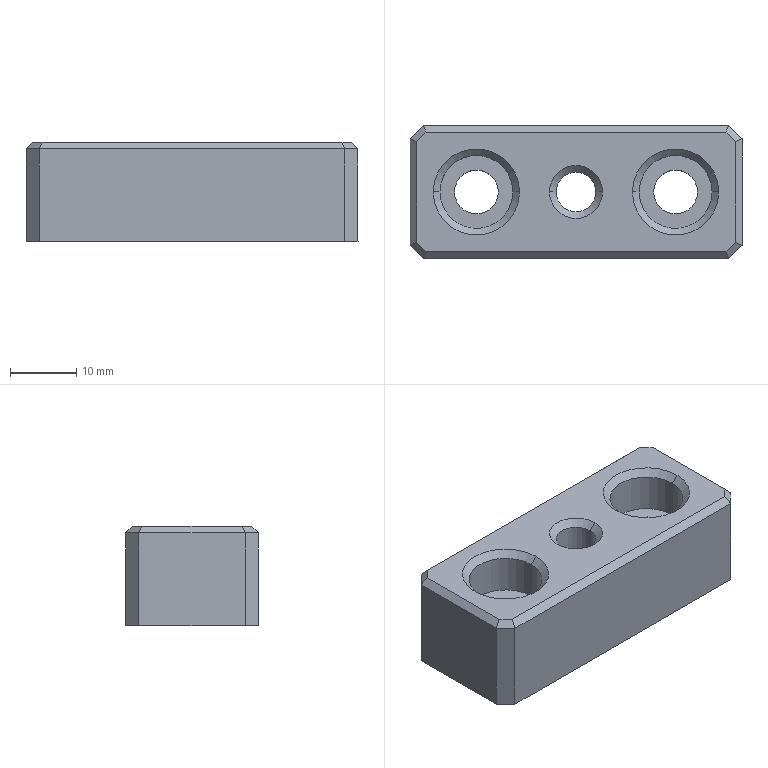Part | SolidWorks | features BaseBody 1 | 1 solid | 36 faces | box 50 x 20 x 15 mm | volume 12489 mm3 | plane 20 | cylinder 10 | cone 6 | commonest cylinder face diameters 6.6 x4 11 x4 6 x2
STEP:
#1=CARTESIAN_POINT('',(360.247,467.,-346.345));
#2=VERTEX_POINT('',#1);
#3=CARTESIAN_POINT('',(354.247,467.,-346.345));
#4=VERTEX_POINT('',#3);
#5=CARTESIAN_POINT('',(357.247,467.,-346.345));
#6=DIRECTION('',(0.,0.,-1.));
#7=DIRECTION('',(-1.,0.,0.));
#8=AXIS2_PLACEMENT_3D('',#5,#6,#7);
#9=CIRCLE('',#8,3.);
#10=EDGE_CURVE('',#2,#4,#9,.T.);
#11=ORIENTED_EDGE('',*,*,#10,.F.);
#12=CARTESIAN_POINT('',(360.247,467.,-360.345));
#13=VERTEX_POINT('',#12);
#14=CARTESIAN_POINT('',(360.247,467.,-360.345));
#15=DIRECTION('',(0.,0.,-1.));
#16=VECTOR('',#15,1000.);
#17=LINE('',#14,#16);
#18=EDGE_CURVE('',#2,#13,#17,.T.);
#19=ORIENTED_EDGE('',*,*,#18,.T.);
#20=CARTESIAN_POINT('',(354.247,467.,-360.345));
#21=VERTEX_POINT('',#20);
#22=CARTESIAN_POINT('',(357.247,467.,-360.345));
#23=DIRECTION('',(0.,0.,-1.));
#24=DIRECTION('',(-1.,0.,0.));
#25=AXIS2_PLACEMENT_3D('',#22,#23,#24);
#26=CIRCLE('',#25,3.);
#27=EDGE_CURVE('',#13,#21,#26,.T.);
#28=ORIENTED_EDGE('',*,*,#27,.T.);
#29=CARTESIAN_POINT('',(354.247,467.,-360.345));
#30=DIRECTION('',(0.,0.,-1.));
#31=VECTOR('',#30,1000.);
#32=LINE('',#29,#31);
#33=EDGE_CURVE('',#4,#21,#32,.T.);
#34=ORIENTED_EDGE('',*,*,#33,.F.);
#35=EDGE_LOOP('',(#11,#19,#28,#34));
#36=FACE_OUTER_BOUND('',#35,.T.);
#37=CARTESIAN_POINT('',(357.247,467.,-360.345));
#38=DIRECTION('',(0.,0.,-1.));
#39=DIRECTION('',(-1.,0.,0.));
#40=AXIS2_PLACEMENT_3D('',#37,#38,#39);
#41=CYLINDRICAL_SURFACE('',#40,3.);
#42=ADVANCED_FACE('',(#36),#41,.F.);
#43=CARTESIAN_POINT('',(345.547,467.,-360.345));
#44=VERTEX_POINT('',#43);
#45=CARTESIAN_POINT('',(338.947,467.,-360.345));
#46=VERTEX_POINT('',#45);
#47=CARTESIAN_POINT('',(342.247,467.,-360.345));
#48=DIRECTION('',(0.,0.,-1.));
#49=DIRECTION('',(1.,0.,0.));
#50=AXIS2_PLACEMENT_3D('',#47,#48,#49);
#51=CIRCLE('',#50,3.3);
#52=EDGE_CURVE('',#44,#46,#51,.T.);
#53=ORIENTED_EDGE('',*,*,#52,.T.);
#54=CARTESIAN_POINT('',(338.947,467.,-352.145));
#55=VERTEX_POINT('',#54);
#56=CARTESIAN_POINT('',(338.947,467.,-345.345));
#57=DIRECTION('',(0.,0.,1.));
#58=VECTOR('',#57,1000.);
#59=LINE('',#56,#58);
#60=EDGE_CURVE('',#46,#55,#59,.T.);
#61=ORIENTED_EDGE('',*,*,#60,.T.);
#62=CARTESIAN_POINT('',(345.547,467.,-352.145));
#63=VERTEX_POINT('',#62);
#64=CARTESIAN_POINT('',(342.247,467.,-352.145));
#65=DIRECTION('',(0.,0.,-1.));
#66=DIRECTION('',(1.,0.,0.));
#67=AXIS2_PLACEMENT_3D('',#64,#65,#66);
#68=CIRCLE('',#67,3.3);
#69=EDGE_CURVE('',#63,#55,#68,.T.);
#70=ORIENTED_EDGE('',*,*,#69,.F.);
#71=CARTESIAN_POINT('',(345.547,467.,-345.345));
#72=DIRECTION('',(0.,0.,1.));
#73=VECTOR('',#72,1000.);
#74=LINE('',#71,#73);
#75=EDGE_CURVE('',#44,#63,#74,.T.);
#76=ORIENTED_EDGE('',*,*,#75,.F.);
#77=EDGE_LOOP('',(#53,#61,#70,#76));
#78=FACE_OUTER_BOUND('',#77,.T.);
#79=CARTESIAN_POINT('',(342.247,467.,-345.345));
#80=DIRECTION('',(0.,0.,1.));
#81=DIRECTION('',(1.,0.,0.));
#82=AXIS2_PLACEMENT_3D('',#79,#80,#81);
#83=CYLINDRICAL_SURFACE('',#82,3.3);
#84=ADVANCED_FACE('',(#78),#83,.F.);
#85=CARTESIAN_POINT('',(375.547,467.,-360.345));
#86=VERTEX_POINT('',#85);
#87=CARTESIAN_POINT('',(368.947,467.,-360.345));
#88=VERTEX_POINT('',#87);
#89=CARTESIAN_POINT('',(372.247,467.,-360.345));
#90=DIRECTION('',(0.,0.,-1.));
#91=DIRECTION('',(1.,0.,0.));
#92=AXIS2_PLACEMENT_3D('',#89,#90,#91);
#93=CIRCLE('',#92,3.3);
#94=EDGE_CURVE('',#86,#88,#93,.T.);
#95=ORIENTED_EDGE('',*,*,#94,.T.);
#96=CARTESIAN_POINT('',(368.947,467.,-352.145));
#97=VERTEX_POINT('',#96);
#98=CARTESIAN_POINT('',(368.947,467.,-345.345));
#99=DIRECTION('',(0.,0.,1.));
#100=VECTOR('',#99,1000.);
#101=LINE('',#98,#100);
#102=EDGE_CURVE('',#88,#97,#101,.T.);
#103=ORIENTED_EDGE('',*,*,#102,.T.);
#104=CARTESIAN_POINT('',(375.547,467.,-352.145));
#105=VERTEX_POINT('',#104);
#106=CARTESIAN_POINT('',(372.247,467.,-352.145));
#107=DIRECTION('',(0.,0.,-1.));
#108=DIRECTION('',(1.,0.,0.));
#109=AXIS2_PLACEMENT_3D('',#106,#107,#108);
#110=CIRCLE('',#109,3.3);
#111=EDGE_CURVE('',#105,#97,#110,.T.);
#112=ORIENTED_EDGE('',*,*,#111,.F.);
#113=CARTESIAN_POINT('',(375.547,467.,-345.345));
#114=DIRECTION('',(0.,0.,1.));
#115=VECTOR('',#114,1000.);
#116=LINE('',#113,#115);
#117=EDGE_CURVE('',#86,#105,#116,.T.);
#118=ORIENTED_EDGE('',*,*,#117,.F.);
#119=EDGE_LOOP('',(#95,#103,#112,#118));
#120=FACE_OUTER_BOUND('',#119,.T.);
#121=CARTESIAN_POINT('',(372.247,467.,-345.345));
#122=DIRECTION('',(0.,0.,1.));
#123=DIRECTION('',(1.,0.,0.));
#124=AXIS2_PLACEMENT_3D('',#121,#122,#123);
#125=CYLINDRICAL_SURFACE('',#124,3.3);
#126=ADVANCED_FACE('',(#120),#125,.F.);
#127=ORIENTED_EDGE('',*,*,#10,.T.);
#128=CARTESIAN_POINT('',(353.247,467.,-345.345));
#129=VERTEX_POINT('',#128);
#130=CARTESIAN_POINT('',(353.247,467.,-345.345));
#131=DIRECTION('',(-0.7071,0.,0.7071));
#132=VECTOR('',#131,1000.);
#133=LINE('',#130,#132);
#134=EDGE_CURVE('',#4,#129,#133,.T.);
#135=ORIENTED_EDGE('',*,*,#134,.T.);
#136=CARTESIAN_POINT('',(361.247,467.,-345.345));
#137=VERTEX_POINT('',#136);
#138=CARTESIAN_POINT('',(357.247,467.,-345.345));
#139=DIRECTION('',(0.,0.,-1.));
#140=DIRECTION('',(1.,0.,0.));
#141=AXIS2_PLACEMENT_3D('',#138,#139,#140);
#142=CIRCLE('',#141,4.);
#143=EDGE_CURVE('',#137,#129,#142,.T.);
#144=ORIENTED_EDGE('',*,*,#143,.F.);
#145=CARTESIAN_POINT('',(361.247,467.,-345.345));
#146=DIRECTION('',(0.7071,0.,0.7071));
#147=VECTOR('',#146,1000.);
#148=LINE('',#145,#147);
#149=EDGE_CURVE('',#2,#137,#148,.T.);
#150=ORIENTED_EDGE('',*,*,#149,.F.);
#151=EDGE_LOOP('',(#127,#135,#144,#150));
#152=FACE_OUTER_BOUND('',#151,.T.);
#153=CARTESIAN_POINT('',(357.247,467.,-345.345));
#154=DIRECTION('',(0.,0.,1.));
#155=DIRECTION('',(1.,0.,0.));
#156=AXIS2_PLACEMENT_3D('',#153,#154,#155);
#157=CONICAL_SURFACE('',#156,4.,0.7854);
#158=ADVANCED_FACE('',(#152),#157,.F.);
#159=CARTESIAN_POINT('',(347.747,467.,-352.145));
#160=VERTEX_POINT('',#159);
#161=CARTESIAN_POINT('',(336.747,467.,-352.145));
#162=VERTEX_POINT('',#161);
#163=CARTESIAN_POINT('',(342.247,467.,-352.145));
#164=DIRECTION('',(0.,0.,-1.));
#165=DIRECTION('',(1.,0.,0.));
#166=AXIS2_PLACEMENT_3D('',#163,#164,#165);
#167=CIRCLE('',#166,5.5);
#168=EDGE_CURVE('',#160,#162,#167,.T.);
#169=ORIENTED_EDGE('',*,*,#168,.T.);
#170=CARTESIAN_POINT('',(336.747,467.,-346.345));
#171=VERTEX_POINT('',#170);
#172=CARTESIAN_POINT('',(336.747,467.,-345.345));
#173=DIRECTION('',(0.,0.,1.));
#174=VECTOR('',#173,1000.);
#175=LINE('',#172,#174);
#176=EDGE_CURVE('',#162,#171,#175,.T.);
#177=ORIENTED_EDGE('',*,*,#176,.T.);
#178=CARTESIAN_POINT('',(347.747,467.,-346.345));
#179=VERTEX_POINT('',#178);
#180=CARTESIAN_POINT('',(342.247,467.,-346.345));
#181=DIRECTION('',(0.,0.,-1.));
#182=DIRECTION('',(1.,0.,0.));
#183=AXIS2_PLACEMENT_3D('',#180,#181,#182);
#184=CIRCLE('',#183,5.5);
#185=EDGE_CURVE('',#179,#171,#184,.T.);
#186=ORIENTED_EDGE('',*,*,#185,.F.);
#187=CARTESIAN_POINT('',(347.747,467.,-345.345));
#188=DIRECTION('',(0.,0.,1.));
#189=VECTOR('',#188,1000.);
#190=LINE('',#187,#189);
#191=EDGE_CURVE('',#160,#179,#190,.T.);
#192=ORIENTED_EDGE('',*,*,#191,.F.);
#193=EDGE_LOOP('',(#169,#177,#186,#192));
#194=FACE_OUTER_BOUND('',#193,.T.);
#195=CARTESIAN_POINT('',(342.247,467.,-345.345));
#196=DIRECTION('',(0.,0.,1.));
#197=DIRECTION('',(1.,0.,0.));
#198=AXIS2_PLACEMENT_3D('',#195,#196,#197);
#199=CYLINDRICAL_SURFACE('',#198,5.5);
#200=ADVANCED_FACE('',(#194),#199,.F.);
#201=CARTESIAN_POINT('',(377.747,467.,-352.145));
#202=VERTEX_POINT('',#201);
#203=CARTESIAN_POINT('',(366.747,467.,-352.145));
#204=VERTEX_POINT('',#203);
#205=CARTESIAN_POINT('',(372.247,467.,-352.145));
#206=DIRECTION('',(0.,0.,-1.));
#207=DIRECTION('',(1.,0.,0.));
#208=AXIS2_PLACEMENT_3D('',#205,#206,#207);
#209=CIRCLE('',#208,5.5);
#210=EDGE_CURVE('',#202,#204,#209,.T.);
#211=ORIENTED_EDGE('',*,*,#210,.T.);
#212=CARTESIAN_POINT('',(366.747,467.,-346.345));
#213=VERTEX_POINT('',#212);
#214=CARTESIAN_POINT('',(366.747,467.,-345.345));
#215=DIRECTION('',(0.,0.,1.));
#216=VECTOR('',#215,1000.);
#217=LINE('',#214,#216);
#218=EDGE_CURVE('',#204,#213,#217,.T.);
#219=ORIENTED_EDGE('',*,*,#218,.T.);
#220=CARTESIAN_POINT('',(377.747,467.,-346.345));
#221=VERTEX_POINT('',#220);
#222=CARTESIAN_POINT('',(372.247,467.,-346.345));
#223=DIRECTION('',(0.,0.,-1.));
#224=DIRECTION('',(1.,0.,0.));
#225=AXIS2_PLACEMENT_3D('',#222,#223,#224);
#226=CIRCLE('',#225,5.5);
#227=EDGE_CURVE('',#221,#213,#226,.T.);
#228=ORIENTED_EDGE('',*,*,#227,.F.);
#229=CARTESIAN_POINT('',(377.747,467.,-345.345));
#230=DIRECTION('',(0.,0.,1.));
#231=VECTOR('',#230,1000.);
#232=LINE('',#229,#231);
#233=EDGE_CURVE('',#202,#221,#232,.T.);
#234=ORIENTED_EDGE('',*,*,#233,.F.);
#235=EDGE_LOOP('',(#211,#219,#228,#234));
#236=FACE_OUTER_BOUND('',#235,.T.);
#237=CARTESIAN_POINT('',(372.247,467.,-345.345));
#238=DIRECTION('',(0.,0.,1.));
#239=DIRECTION('',(1.,0.,0.));
#240=AXIS2_PLACEMENT_3D('',#237,#238,#239);
#241=CYLINDRICAL_SURFACE('',#240,5.5);
#242=ADVANCED_FACE('',(#236),#241,.F.);
#243=ORIENTED_EDGE('',*,*,#227,.T.);
#244=CARTESIAN_POINT('',(365.747,467.,-345.345));
#245=VERTEX_POINT('',#244);
#246=CARTESIAN_POINT('',(365.747,467.,-345.345));
#247=DIRECTION('',(-0.7071,0.,0.7071));
#248=VECTOR('',#247,1000.);
#249=LINE('',#246,#248);
#250=EDGE_CURVE('',#213,#245,#249,.T.);
#251=ORIENTED_EDGE('',*,*,#250,.T.);
#252=CARTESIAN_POINT('',(378.747,467.,-345.345));
#253=VERTEX_POINT('',#252);
#254=CARTESIAN_POINT('',(372.247,467.,-345.345));
#255=DIRECTION('',(0.,0.,-1.));
#256=DIRECTION('',(1.,0.,0.));
#257=AXIS2_PLACEMENT_3D('',#254,#255,#256);
#258=CIRCLE('',#257,6.5);
#259=EDGE_CURVE('',#253,#245,#258,.T.);
#260=ORIENTED_EDGE('',*,*,#259,.F.);
#261=CARTESIAN_POINT('',(378.747,467.,-345.345));
#262=DIRECTION('',(0.7071,0.,0.7071));
#263=VECTOR('',#262,1000.);
#264=LINE('',#261,#263);
#265=EDGE_CURVE('',#221,#253,#264,.T.);
#266=ORIENTED_EDGE('',*,*,#265,.F.);
#267=EDGE_LOOP('',(#243,#251,#260,#266));
#268=FACE_OUTER_BOUND('',#267,.T.);
#269=CARTESIAN_POINT('',(372.247,467.,-345.345));
#270=DIRECTION('',(0.,0.,1.));
#271=DIRECTION('',(1.,0.,0.));
#272=AXIS2_PLACEMENT_3D('',#269,#270,#271);
#273=CONICAL_SURFACE('',#272,6.5,0.7854);
#274=ADVANCED_FACE('',(#268),#273,.F.);
#275=ORIENTED_EDGE('',*,*,#185,.T.);
#276=CARTESIAN_POINT('',(335.747,467.,-345.345));
#277=VERTEX_POINT('',#276);
#278=CARTESIAN_POINT('',(335.747,467.,-345.345));
#279=DIRECTION('',(-0.7071,0.,0.7071));
#280=VECTOR('',#279,1000.);
#281=LINE('',#278,#280);
#282=EDGE_CURVE('',#171,#277,#281,.T.);
#283=ORIENTED_EDGE('',*,*,#282,.T.);
#284=CARTESIAN_POINT('',(348.747,467.,-345.345));
#285=VERTEX_POINT('',#284);
#286=CARTESIAN_POINT('',(342.247,467.,-345.345));
#287=DIRECTION('',(0.,0.,-1.));
#288=DIRECTION('',(1.,0.,0.));
#289=AXIS2_PLACEMENT_3D('',#286,#287,#288);
#290=CIRCLE('',#289,6.5);
#291=EDGE_CURVE('',#285,#277,#290,.T.);
#292=ORIENTED_EDGE('',*,*,#291,.F.);
#293=CARTESIAN_POINT('',(348.747,467.,-345.345));
#294=DIRECTION('',(0.7071,0.,0.7071));
#295=VECTOR('',#294,1000.);
#296=LINE('',#293,#295);
#297=EDGE_CURVE('',#179,#285,#296,.T.);
#298=ORIENTED_EDGE('',*,*,#297,.F.);
#299=EDGE_LOOP('',(#275,#283,#292,#298));
#300=FACE_OUTER_BOUND('',#299,.T.);
#301=CARTESIAN_POINT('',(342.247,467.,-345.345));
#302=DIRECTION('',(0.,0.,1.));
#303=DIRECTION('',(1.,0.,0.));
#304=AXIS2_PLACEMENT_3D('',#301,#302,#303);
#305=CONICAL_SURFACE('',#304,6.5,0.7854);
#306=ADVANCED_FACE('',(#300),#305,.F.);
#307=CARTESIAN_POINT('',(357.247,467.,-360.345));
#308=DIRECTION('',(0.,0.,-1.));
#309=DIRECTION('',(-1.,0.,0.));
#310=AXIS2_PLACEMENT_3D('',#307,#308,#309);
#311=CIRCLE('',#310,3.);
#312=EDGE_CURVE('',#21,#13,#311,.T.);
#313=ORIENTED_EDGE('',*,*,#312,.F.);
#314=ORIENTED_EDGE('',*,*,#27,.F.);
#315=EDGE_LOOP('',(#313,#314));
#316=FACE_BOUND('',#315,.T.);
#317=ORIENTED_EDGE('',*,*,#52,.F.);
#318=CARTESIAN_POINT('',(342.247,467.,-360.345));
#319=DIRECTION('',(0.,0.,-1.));
#320=DIRECTION('',(1.,0.,0.));
#321=AXIS2_PLACEMENT_3D('',#318,#319,#320);
#322=CIRCLE('',#321,3.3);
#323=EDGE_CURVE('',#46,#44,#322,.T.);
#324=ORIENTED_EDGE('',*,*,#323,.F.);
#325=EDGE_LOOP('',(#317,#324));
#326=FACE_BOUND('',#325,.T.);
#327=ORIENTED_EDGE('',*,*,#94,.F.);
#328=CARTESIAN_POINT('',(372.247,467.,-360.345));
#329=DIRECTION('',(0.,0.,-1.));
#330=DIRECTION('',(1.,0.,0.));
#331=AXIS2_PLACEMENT_3D('',#328,#329,#330);
#332=CIRCLE('',#331,3.3);
#333=EDGE_CURVE('',#88,#86,#332,.T.);
#334=ORIENTED_EDGE('',*,*,#333,.F.);
#335=EDGE_LOOP('',(#327,#334));
#336=FACE_BOUND('',#335,.T.);
#337=CARTESIAN_POINT('',(332.247,475.,-360.345));
#338=VERTEX_POINT('',#337);
#339=CARTESIAN_POINT('',(332.247,459.,-360.345));
#340=VERTEX_POINT('',#339);
#341=CARTESIAN_POINT('',(332.247,467.,-360.345));
#342=DIRECTION('',(0.,-1.,0.));
#343=VECTOR('',#342,1000.);
#344=LINE('',#341,#343);
#345=EDGE_CURVE('',#338,#340,#344,.T.);
#346=ORIENTED_EDGE('',*,*,#345,.F.);
#347=CARTESIAN_POINT('',(334.247,477.,-360.345));
#348=VERTEX_POINT('',#347);
#349=CARTESIAN_POINT('',(334.247,477.,-360.345));
#350=DIRECTION('',(-0.7071,-0.7071,0.));
#351=VECTOR('',#350,1000.);
#352=LINE('',#349,#351);
#353=EDGE_CURVE('',#348,#338,#352,.T.);
#354=ORIENTED_EDGE('',*,*,#353,.F.);
#355=CARTESIAN_POINT('',(380.247,477.,-360.345));
#356=VERTEX_POINT('',#355);
#357=CARTESIAN_POINT('',(357.247,477.,-360.345));
#358=DIRECTION('',(-1.,0.,0.));
#359=VECTOR('',#358,1000.);
#360=LINE('',#357,#359);
#361=EDGE_CURVE('',#356,#348,#360,.T.);
#362=ORIENTED_EDGE('',*,*,#361,.F.);
#363=CARTESIAN_POINT('',(382.247,475.,-360.345));
#364=VERTEX_POINT('',#363);
#365=CARTESIAN_POINT('',(382.247,475.,-360.345));
#366=DIRECTION('',(-0.7071,0.7071,0.));
#367=VECTOR('',#366,1000.);
#368=LINE('',#365,#367);
#369=EDGE_CURVE('',#364,#356,#368,.T.);
#370=ORIENTED_EDGE('',*,*,#369,.F.);
#371=CARTESIAN_POINT('',(382.247,459.,-360.345));
#372=VERTEX_POINT('',#371);
#373=CARTESIAN_POINT('',(382.247,467.,-360.345));
#374=DIRECTION('',(0.,1.,0.));
#375=VECTOR('',#374,1000.);
#376=LINE('',#373,#375);
#377=EDGE_CURVE('',#372,#364,#376,.T.);
#378=ORIENTED_EDGE('',*,*,#377,.F.);
#379=CARTESIAN_POINT('',(380.247,457.,-360.345));
#380=VERTEX_POINT('',#379);
#381=CARTESIAN_POINT('',(380.247,457.,-360.345));
#382=DIRECTION('',(0.7071,0.7071,0.));
#383=VECTOR('',#382,1000.);
#384=LINE('',#381,#383);
#385=EDGE_CURVE('',#380,#372,#384,.T.);
#386=ORIENTED_EDGE('',*,*,#385,.F.);
#387=CARTESIAN_POINT('',(334.247,457.,-360.345));
#388=VERTEX_POINT('',#387);
#389=CARTESIAN_POINT('',(357.247,457.,-360.345));
#390=DIRECTION('',(1.,0.,0.));
#391=VECTOR('',#390,1000.);
#392=LINE('',#389,#391);
#393=EDGE_CURVE('',#388,#380,#392,.T.);
#394=ORIENTED_EDGE('',*,*,#393,.F.);
#395=CARTESIAN_POINT('',(332.247,459.,-360.345));
#396=DIRECTION('',(0.7071,-0.7071,0.));
#397=VECTOR('',#396,1000.);
#398=LINE('',#395,#397);
#399=EDGE_CURVE('',#340,#388,#398,.T.);
#400=ORIENTED_EDGE('',*,*,#399,.F.);
#401=EDGE_LOOP('',(#346,#354,#362,#370,#378,#386,#394,#400));
#402=FACE_OUTER_BOUND('',#401,.T.);
#403=CARTESIAN_POINT('',(357.247,467.,-360.345));
#404=DIRECTION('',(0.,0.,1.));
#405=DIRECTION('',(1.,0.,0.));
#406=AXIS2_PLACEMENT_3D('',#403,#404,#405);
#407=PLANE('',#406);
#408=ADVANCED_FACE('',(#316,#326,#336,#402),#407,.F.);
#409=ORIENTED_EDGE('',*,*,#18,.F.);
#410=CARTESIAN_POINT('',(357.247,467.,-346.345));
#411=DIRECTION('',(0.,0.,-1.));
#412=DIRECTION('',(-1.,0.,0.));
#413=AXIS2_PLACEMENT_3D('',#410,#411,#412);
#414=CIRCLE('',#413,3.);
#415=EDGE_CURVE('',#4,#2,#414,.T.);
#416=ORIENTED_EDGE('',*,*,#415,.F.);
#417=ORIENTED_EDGE('',*,*,#33,.T.);
#418=ORIENTED_EDGE('',*,*,#312,.T.);
#419=EDGE_LOOP('',(#409,#416,#417,#418));
#420=FACE_OUTER_BOUND('',#419,.T.);
#421=CARTESIAN_POINT('',(357.247,467.,-360.345));
#422=DIRECTION('',(0.,0.,-1.));
#423=DIRECTION('',(-1.,0.,0.));
#424=AXIS2_PLACEMENT_3D('',#421,#422,#423);
#425=CYLINDRICAL_SURFACE('',#424,3.);
#426=ADVANCED_FACE('',(#420),#425,.F.);
#427=ORIENTED_EDGE('',*,*,#60,.F.);
#428=ORIENTED_EDGE('',*,*,#323,.T.);
#429=ORIENTED_EDGE('',*,*,#75,.T.);
#430=CARTESIAN_POINT('',(342.247,467.,-352.145));
#431=DIRECTION('',(0.,0.,-1.));
#432=DIRECTION('',(1.,0.,0.));
#433=AXIS2_PLACEMENT_3D('',#430,#431,#432);
#434=CIRCLE('',#433,3.3);
#435=EDGE_CURVE('',#55,#63,#434,.T.);
#436=ORIENTED_EDGE('',*,*,#435,.F.);
#437=EDGE_LOOP('',(#427,#428,#429,#436));
#438=FACE_OUTER_BOUND('',#437,.T.);
#439=CARTESIAN_POINT('',(342.247,467.,-345.345));
#440=DIRECTION('',(0.,0.,1.));
#441=DIRECTION('',(1.,0.,0.));
#442=AXIS2_PLACEMENT_3D('',#439,#440,#441);
#443=CYLINDRICAL_SURFACE('',#442,3.3);
#444=ADVANCED_FACE('',(#438),#443,.F.);
#445=ORIENTED_EDGE('',*,*,#102,.F.);
#446=ORIENTED_EDGE('',*,*,#333,.T.);
#447=ORIENTED_EDGE('',*,*,#117,.T.);
#448=CARTESIAN_POINT('',(372.247,467.,-352.145));
#449=DIRECTION('',(0.,0.,-1.));
#450=DIRECTION('',(1.,0.,0.));
#451=AXIS2_PLACEMENT_3D('',#448,#449,#450);
#452=CIRCLE('',#451,3.3);
#453=EDGE_CURVE('',#97,#105,#452,.T.);
#454=ORIENTED_EDGE('',*,*,#453,.F.);
#455=EDGE_LOOP('',(#445,#446,#447,#454));
#456=FACE_OUTER_BOUND('',#455,.T.);
#457=CARTESIAN_POINT('',(372.247,467.,-345.345));
#458=DIRECTION('',(0.,0.,1.));
#459=DIRECTION('',(1.,0.,0.));
#460=AXIS2_PLACEMENT_3D('',#457,#458,#459);
#461=CYLINDRICAL_SURFACE('',#460,3.3);
#462=ADVANCED_FACE('',(#456),#461,.F.);
#463=CARTESIAN_POINT('',(332.247,459.,-346.345));
#464=VERTEX_POINT('',#463);
#465=CARTESIAN_POINT('',(332.247,459.,-345.345));
#466=DIRECTION('',(0.,0.,1.));
#467=VECTOR('',#466,1000.);
#468=LINE('',#465,#467);
#469=EDGE_CURVE('',#340,#464,#468,.T.);
#470=ORIENTED_EDGE('',*,*,#469,.F.);
#471=ORIENTED_EDGE('',*,*,#399,.T.);
#472=CARTESIAN_POINT('',(334.247,457.,-346.345));
#473=VERTEX_POINT('',#472);
#474=CARTESIAN_POINT('',(334.247,457.,-345.345));
#475=DIRECTION('',(0.,0.,-1.));
#476=VECTOR('',#475,1000.);
#477=LINE('',#474,#476);
#478=EDGE_CURVE('',#473,#388,#477,.T.);
#479=ORIENTED_EDGE('',*,*,#478,.F.);
#480=CARTESIAN_POINT('',(334.247,457.,-346.345));
#481=DIRECTION('',(0.7071,-0.7071,0.));
#482=VECTOR('',#481,1000.);
#483=LINE('',#480,#482);
#484=EDGE_CURVE('',#464,#473,#483,.T.);
#485=ORIENTED_EDGE('',*,*,#484,.F.);
#486=EDGE_LOOP('',(#470,#471,#479,#485));
#487=FACE_OUTER_BOUND('',#486,.T.);
#488=CARTESIAN_POINT('',(334.247,457.,-345.345));
#489=DIRECTION('',(0.7071,0.7071,0.));
#490=DIRECTION('',(-0.7071,0.7071,0.));
#491=AXIS2_PLACEMENT_3D('',#488,#489,#490);
#492=PLANE('',#491);
#493=ADVANCED_FACE('',(#487),#492,.F.);
#494=CARTESIAN_POINT('',(332.247,475.,-346.345));
#495=VERTEX_POINT('',#494);
#496=CARTESIAN_POINT('',(332.247,475.,-345.345));
#497=DIRECTION('',(0.,0.,1.));
#498=VECTOR('',#497,1000.);
#499=LINE('',#496,#498);
#500=EDGE_CURVE('',#338,#495,#499,.T.);
#501=ORIENTED_EDGE('',*,*,#500,.F.);
#502=ORIENTED_EDGE('',*,*,#345,.T.);
#503=ORIENTED_EDGE('',*,*,#469,.T.);
#504=CARTESIAN_POINT('',(332.247,457.,-346.345));
#505=DIRECTION('',(0.,-1.,0.));
#506=VECTOR('',#505,1000.);
#507=LINE('',#504,#506);
#508=EDGE_CURVE('',#495,#464,#507,.T.);
#509=ORIENTED_EDGE('',*,*,#508,.F.);
#510=EDGE_LOOP('',(#501,#502,#503,#509));
#511=FACE_OUTER_BOUND('',#510,.T.);
#512=CARTESIAN_POINT('',(332.247,457.,-345.345));
#513=DIRECTION('',(1.,0.,0.));
#514=DIRECTION('',(0.,0.,-1.));
#515=AXIS2_PLACEMENT_3D('',#512,#513,#514);
#516=PLANE('',#515);
#517=ADVANCED_FACE('',(#511),#516,.F.);
#518=CARTESIAN_POINT('',(334.247,477.,-346.345));
#519=VERTEX_POINT('',#518);
#520=CARTESIAN_POINT('',(334.247,477.,-345.345));
#521=DIRECTION('',(0.,0.,1.));
#522=VECTOR('',#521,1000.);
#523=LINE('',#520,#522);
#524=EDGE_CURVE('',#348,#519,#523,.T.);
#525=ORIENTED_EDGE('',*,*,#524,.F.);
#526=ORIENTED_EDGE('',*,*,#353,.T.);
#527=ORIENTED_EDGE('',*,*,#500,.T.);
#528=CARTESIAN_POINT('',(332.247,475.,-346.345));
#529=DIRECTION('',(-0.7071,-0.7071,0.));
#530=VECTOR('',#529,1000.);
#531=LINE('',#528,#530);
#532=EDGE_CURVE('',#519,#495,#531,.T.);
#533=ORIENTED_EDGE('',*,*,#532,.F.);
#534=EDGE_LOOP('',(#525,#526,#527,#533));
#535=FACE_OUTER_BOUND('',#534,.T.);
#536=CARTESIAN_POINT('',(332.247,475.,-345.345));
#537=DIRECTION('',(0.7071,-0.7071,0.));
#538=DIRECTION('',(0.7071,0.7071,0.));
#539=AXIS2_PLACEMENT_3D('',#536,#537,#538);
#540=PLANE('',#539);
#541=ADVANCED_FACE('',(#535),#540,.F.);
#542=CARTESIAN_POINT('',(380.247,477.,-346.345));
#543=VERTEX_POINT('',#542);
#544=CARTESIAN_POINT('',(380.247,477.,-345.345));
#545=DIRECTION('',(0.,0.,1.));
#546=VECTOR('',#545,1000.);
#547=LINE('',#544,#546);
#548=EDGE_CURVE('',#356,#543,#547,.T.);
#549=ORIENTED_EDGE('',*,*,#548,.F.);
#550=ORIENTED_EDGE('',*,*,#361,.T.);
#551=ORIENTED_EDGE('',*,*,#524,.T.);
#552=CARTESIAN_POINT('',(332.247,477.,-346.345));
#553=DIRECTION('',(-1.,0.,0.));
#554=VECTOR('',#553,1000.);
#555=LINE('',#552,#554);
#556=EDGE_CURVE('',#543,#519,#555,.T.);
#557=ORIENTED_EDGE('',*,*,#556,.F.);
#558=EDGE_LOOP('',(#549,#550,#551,#557));
#559=FACE_OUTER_BOUND('',#558,.T.);
#560=CARTESIAN_POINT('',(332.247,477.,-345.345));
#561=DIRECTION('',(0.,-1.,0.));
#562=DIRECTION('',(0.,0.,-1.));
#563=AXIS2_PLACEMENT_3D('',#560,#561,#562);
#564=PLANE('',#563);
#565=ADVANCED_FACE('',(#559),#564,.F.);
#566=CARTESIAN_POINT('',(382.247,475.,-346.345));
#567=VERTEX_POINT('',#566);
#568=CARTESIAN_POINT('',(382.247,475.,-345.345));
#569=DIRECTION('',(0.,0.,1.));
#570=VECTOR('',#569,1000.);
#571=LINE('',#568,#570);
#572=EDGE_CURVE('',#364,#567,#571,.T.);
#573=ORIENTED_EDGE('',*,*,#572,.F.);
#574=ORIENTED_EDGE('',*,*,#369,.T.);
#575=ORIENTED_EDGE('',*,*,#548,.T.);
#576=CARTESIAN_POINT('',(380.247,477.,-346.345));
#577=DIRECTION('',(-0.7071,0.7071,0.));
#578=VECTOR('',#577,1000.);
#579=LINE('',#576,#578);
#580=EDGE_CURVE('',#567,#543,#579,.T.);
#581=ORIENTED_EDGE('',*,*,#580,.F.);
#582=EDGE_LOOP('',(#573,#574,#575,#581));
#583=FACE_OUTER_BOUND('',#582,.T.);
#584=CARTESIAN_POINT('',(380.247,477.,-345.345));
#585=DIRECTION('',(-0.7071,-0.7071,0.));
#586=DIRECTION('',(0.7071,-0.7071,0.));
#587=AXIS2_PLACEMENT_3D('',#584,#585,#586);
#588=PLANE('',#587);
#589=ADVANCED_FACE('',(#583),#588,.F.);
#590=CARTESIAN_POINT('',(382.247,459.,-346.345));
#591=VERTEX_POINT('',#590);
#592=CARTESIAN_POINT('',(382.247,459.,-345.345));
#593=DIRECTION('',(0.,0.,1.));
#594=VECTOR('',#593,1000.);
#595=LINE('',#592,#594);
#596=EDGE_CURVE('',#372,#591,#595,.T.);
#597=ORIENTED_EDGE('',*,*,#596,.F.);
#598=ORIENTED_EDGE('',*,*,#377,.T.);
#599=ORIENTED_EDGE('',*,*,#572,.T.);
#600=CARTESIAN_POINT('',(382.247,457.,-346.345));
#601=DIRECTION('',(0.,1.,0.));
#602=VECTOR('',#601,1000.);
#603=LINE('',#600,#602);
#604=EDGE_CURVE('',#591,#567,#603,.T.);
#605=ORIENTED_EDGE('',*,*,#604,.F.);
#606=EDGE_LOOP('',(#597,#598,#599,#605));
#607=FACE_OUTER_BOUND('',#606,.T.);
#608=CARTESIAN_POINT('',(382.247,457.,-345.345));
#609=DIRECTION('',(-1.,0.,0.));
#610=DIRECTION('',(0.,0.,1.));
#611=AXIS2_PLACEMENT_3D('',#608,#609,#610);
#612=PLANE('',#611);
#613=ADVANCED_FACE('',(#607),#612,.F.);
#614=CARTESIAN_POINT('',(380.247,457.,-346.345));
#615=VERTEX_POINT('',#614);
#616=CARTESIAN_POINT('',(380.247,457.,-345.345));
#617=DIRECTION('',(0.,0.,1.));
#618=VECTOR('',#617,1000.);
#619=LINE('',#616,#618);
#620=EDGE_CURVE('',#380,#615,#619,.T.);
#621=ORIENTED_EDGE('',*,*,#620,.F.);
#622=ORIENTED_EDGE('',*,*,#385,.T.);
#623=ORIENTED_EDGE('',*,*,#596,.T.);
#624=CARTESIAN_POINT('',(382.247,459.,-346.345));
#625=DIRECTION('',(0.7071,0.7071,0.));
#626=VECTOR('',#625,1000.);
#627=LINE('',#624,#626);
#628=EDGE_CURVE('',#615,#591,#627,.T.);
#629=ORIENTED_EDGE('',*,*,#628,.F.);
#630=EDGE_LOOP('',(#621,#622,#623,#629));
#631=FACE_OUTER_BOUND('',#630,.T.);
#632=CARTESIAN_POINT('',(382.247,459.,-345.345));
#633=DIRECTION('',(-0.7071,0.7071,0.));
#634=DIRECTION('',(-0.7071,-0.7071,0.));
#635=AXIS2_PLACEMENT_3D('',#632,#633,#634);
#636=PLANE('',#635);
#637=ADVANCED_FACE('',(#631),#636,.F.);
#638=ORIENTED_EDGE('',*,*,#478,.T.);
#639=ORIENTED_EDGE('',*,*,#393,.T.);
#640=ORIENTED_EDGE('',*,*,#620,.T.);
#641=CARTESIAN_POINT('',(332.247,457.,-346.345));
#642=DIRECTION('',(1.,0.,0.));
#643=VECTOR('',#642,1000.);
#644=LINE('',#641,#643);
#645=EDGE_CURVE('',#473,#615,#644,.T.);
#646=ORIENTED_EDGE('',*,*,#645,.F.);
#647=EDGE_LOOP('',(#638,#639,#640,#646));
#648=FACE_OUTER_BOUND('',#647,.T.);
#649=CARTESIAN_POINT('',(332.247,457.,-345.345));
#650=DIRECTION('',(0.,1.,0.));
#651=DIRECTION('',(0.,0.,1.));
#652=AXIS2_PLACEMENT_3D('',#649,#650,#651);
#653=PLANE('',#652);
#654=ADVANCED_FACE('',(#648),#653,.F.);
#655=ORIENTED_EDGE('',*,*,#134,.F.);
#656=ORIENTED_EDGE('',*,*,#415,.T.);
#657=ORIENTED_EDGE('',*,*,#149,.T.);
#658=CARTESIAN_POINT('',(357.247,467.,-345.345));
#659=DIRECTION('',(0.,0.,-1.));
#660=DIRECTION('',(1.,0.,0.));
#661=AXIS2_PLACEMENT_3D('',#658,#659,#660);
#662=CIRCLE('',#661,4.);
#663=EDGE_CURVE('',#129,#137,#662,.T.);
#664=ORIENTED_EDGE('',*,*,#663,.F.);
#665=EDGE_LOOP('',(#655,#656,#657,#664));
#666=FACE_OUTER_BOUND('',#665,.T.);
#667=CARTESIAN_POINT('',(357.247,467.,-345.345));
#668=DIRECTION('',(0.,0.,1.));
#669=DIRECTION('',(1.,0.,0.));
#670=AXIS2_PLACEMENT_3D('',#667,#668,#669);
#671=CONICAL_SURFACE('',#670,4.,0.7854);
#672=ADVANCED_FACE('',(#666),#671,.F.);
#673=ORIENTED_EDGE('',*,*,#69,.T.);
#674=ORIENTED_EDGE('',*,*,#435,.T.);
#675=EDGE_LOOP('',(#673,#674));
#676=FACE_BOUND('',#675,.T.);
#677=ORIENTED_EDGE('',*,*,#168,.F.);
#678=CARTESIAN_POINT('',(342.247,467.,-352.145));
#679=DIRECTION('',(0.,0.,-1.));
#680=DIRECTION('',(1.,0.,0.));
#681=AXIS2_PLACEMENT_3D('',#678,#679,#680);
#682=CIRCLE('',#681,5.5);
#683=EDGE_CURVE('',#162,#160,#682,.T.);
#684=ORIENTED_EDGE('',*,*,#683,.F.);
#685=EDGE_LOOP('',(#677,#684));
#686=FACE_OUTER_BOUND('',#685,.T.);
#687=CARTESIAN_POINT('',(342.247,470.3,-352.145));
#688=DIRECTION('',(0.,0.,-1.));
#689=DIRECTION('',(-1.,0.,0.));
#690=AXIS2_PLACEMENT_3D('',#687,#688,#689);
#691=PLANE('',#690);
#692=ADVANCED_FACE('',(#676,#686),#691,.F.);
#693=ORIENTED_EDGE('',*,*,#111,.T.);
#694=ORIENTED_EDGE('',*,*,#453,.T.);
#695=EDGE_LOOP('',(#693,#694));
#696=FACE_BOUND('',#695,.T.);
#697=ORIENTED_EDGE('',*,*,#210,.F.);
#698=CARTESIAN_POINT('',(372.247,467.,-352.145));
#699=DIRECTION('',(0.,0.,-1.));
#700=DIRECTION('',(1.,0.,0.));
#701=AXIS2_PLACEMENT_3D('',#698,#699,#700);
#702=CIRCLE('',#701,5.5);
#703=EDGE_CURVE('',#204,#202,#702,.T.);
#704=ORIENTED_EDGE('',*,*,#703,.F.);
#705=EDGE_LOOP('',(#697,#704));
#706=FACE_OUTER_BOUND('',#705,.T.);
#707=CARTESIAN_POINT('',(372.247,470.3,-352.145));
#708=DIRECTION('',(0.,0.,-1.));
#709=DIRECTION('',(-1.,0.,0.));
#710=AXIS2_PLACEMENT_3D('',#707,#708,#709);
#711=PLANE('',#710);
#712=ADVANCED_FACE('',(#696,#706),#711,.F.);
#713=ORIENTED_EDGE('',*,*,#484,.T.);
#714=CARTESIAN_POINT('',(334.661,458.,-345.345));
#715=VERTEX_POINT('',#714);
#716=CARTESIAN_POINT('',(334.247,457.,-346.345));
#717=DIRECTION('',(0.2811,0.6786,0.6786));
#718=VECTOR('',#717,1000.);
#719=LINE('',#716,#718);
#720=EDGE_CURVE('',#473,#715,#719,.T.);
#721=ORIENTED_EDGE('',*,*,#720,.T.);
#722=CARTESIAN_POINT('',(333.247,459.414,-345.345));
#723=VERTEX_POINT('',#722);
#724=CARTESIAN_POINT('',(334.661,458.,-345.345));
#725=DIRECTION('',(-0.7071,0.7071,0.));
#726=VECTOR('',#725,1000.);
#727=LINE('',#724,#726);
#728=EDGE_CURVE('',#715,#723,#727,.T.);
#729=ORIENTED_EDGE('',*,*,#728,.T.);
#730=CARTESIAN_POINT('',(333.247,459.414,-345.345));
#731=DIRECTION('',(-0.6786,-0.2811,-0.6786));
#732=VECTOR('',#731,1000.);
#733=LINE('',#730,#732);
#734=EDGE_CURVE('',#723,#464,#733,.T.);
#735=ORIENTED_EDGE('',*,*,#734,.T.);
#736=EDGE_LOOP('',(#713,#721,#729,#735));
#737=FACE_OUTER_BOUND('',#736,.T.);
#738=CARTESIAN_POINT('',(341.454,451.207,-345.345));
#739=DIRECTION('',(-0.5,-0.5,0.7071));
#740=DIRECTION('',(0.8165,0.,0.5774));
#741=AXIS2_PLACEMENT_3D('',#738,#739,#740);
#742=PLANE('',#741);
#743=ADVANCED_FACE('',(#737),#742,.T.);
#744=ORIENTED_EDGE('',*,*,#508,.T.);
#745=ORIENTED_EDGE('',*,*,#734,.F.);
#746=CARTESIAN_POINT('',(333.247,474.586,-345.345));
#747=VERTEX_POINT('',#746);
#748=CARTESIAN_POINT('',(333.247,467.,-345.345));
#749=DIRECTION('',(0.,1.,0.));
#750=VECTOR('',#749,1000.);
#751=LINE('',#748,#750);
#752=EDGE_CURVE('',#723,#747,#751,.T.);
#753=ORIENTED_EDGE('',*,*,#752,.T.);
#754=CARTESIAN_POINT('',(333.247,474.586,-345.345));
#755=DIRECTION('',(-0.6786,0.2811,-0.6786));
#756=VECTOR('',#755,1000.);
#757=LINE('',#754,#756);
#758=EDGE_CURVE('',#747,#495,#757,.T.);
#759=ORIENTED_EDGE('',*,*,#758,.T.);
#760=EDGE_LOOP('',(#744,#745,#753,#759));
#761=FACE_OUTER_BOUND('',#760,.T.);
#762=CARTESIAN_POINT('',(333.247,467.,-345.345));
#763=DIRECTION('',(-0.7071,0.,0.7071));
#764=DIRECTION('',(0.7071,0.,0.7071));
#765=AXIS2_PLACEMENT_3D('',#762,#763,#764);
#766=PLANE('',#765);
#767=ADVANCED_FACE('',(#761),#766,.T.);
#768=CARTESIAN_POINT('',(334.661,476.,-345.345));
#769=VERTEX_POINT('',#768);
#770=CARTESIAN_POINT('',(333.247,474.586,-345.345));
#771=DIRECTION('',(0.7071,0.7071,0.));
#772=VECTOR('',#771,1000.);
#773=LINE('',#770,#772);
#774=EDGE_CURVE('',#747,#769,#773,.T.);
#775=ORIENTED_EDGE('',*,*,#774,.T.);
#776=CARTESIAN_POINT('',(334.661,476.,-345.345));
#777=DIRECTION('',(-0.2811,0.6786,-0.6786));
#778=VECTOR('',#777,1000.);
#779=LINE('',#776,#778);
#780=EDGE_CURVE('',#769,#519,#779,.T.);
#781=ORIENTED_EDGE('',*,*,#780,.T.);
#782=ORIENTED_EDGE('',*,*,#532,.T.);
#783=ORIENTED_EDGE('',*,*,#758,.F.);
#784=EDGE_LOOP('',(#775,#781,#782,#783));
#785=FACE_OUTER_BOUND('',#784,.T.);
#786=CARTESIAN_POINT('',(341.454,482.793,-345.345));
#787=DIRECTION('',(-0.5,0.5,0.7071));
#788=DIRECTION('',(0.8165,0.,0.5774));
#789=AXIS2_PLACEMENT_3D('',#786,#787,#788);
#790=PLANE('',#789);
#791=ADVANCED_FACE('',(#785),#790,.T.);
#792=CARTESIAN_POINT('',(379.832,476.,-345.345));
#793=VERTEX_POINT('',#792);
#794=CARTESIAN_POINT('',(357.247,476.,-345.345));
#795=DIRECTION('',(1.,0.,0.));
#796=VECTOR('',#795,1000.);
#797=LINE('',#794,#796);
#798=EDGE_CURVE('',#769,#793,#797,.T.);
#799=ORIENTED_EDGE('',*,*,#798,.T.);
#800=CARTESIAN_POINT('',(379.832,476.,-345.345));
#801=DIRECTION('',(0.2811,0.6786,-0.6786));
#802=VECTOR('',#801,1000.);
#803=LINE('',#800,#802);
#804=EDGE_CURVE('',#793,#543,#803,.T.);
#805=ORIENTED_EDGE('',*,*,#804,.T.);
#806=ORIENTED_EDGE('',*,*,#556,.T.);
#807=ORIENTED_EDGE('',*,*,#780,.F.);
#808=EDGE_LOOP('',(#799,#805,#806,#807));
#809=FACE_OUTER_BOUND('',#808,.T.);
#810=CARTESIAN_POINT('',(357.247,476.,-345.345));
#811=DIRECTION('',(0.,0.7071,0.7071));
#812=DIRECTION('',(0.,-0.7071,0.7071));
#813=AXIS2_PLACEMENT_3D('',#810,#811,#812);
#814=PLANE('',#813);
#815=ADVANCED_FACE('',(#809),#814,.T.);
#816=CARTESIAN_POINT('',(381.247,474.586,-345.345));
#817=VERTEX_POINT('',#816);
#818=CARTESIAN_POINT('',(379.832,476.,-345.345));
#819=DIRECTION('',(0.7071,-0.7071,0.));
#820=VECTOR('',#819,1000.);
#821=LINE('',#818,#820);
#822=EDGE_CURVE('',#793,#817,#821,.T.);
#823=ORIENTED_EDGE('',*,*,#822,.T.);
#824=CARTESIAN_POINT('',(381.247,474.586,-345.345));
#825=DIRECTION('',(0.6786,0.2811,-0.6786));
#826=VECTOR('',#825,1000.);
#827=LINE('',#824,#826);
#828=EDGE_CURVE('',#817,#567,#827,.T.);
#829=ORIENTED_EDGE('',*,*,#828,.T.);
#830=ORIENTED_EDGE('',*,*,#580,.T.);
#831=ORIENTED_EDGE('',*,*,#804,.F.);
#832=EDGE_LOOP('',(#823,#829,#830,#831));
#833=FACE_OUTER_BOUND('',#832,.T.);
#834=CARTESIAN_POINT('',(373.039,482.793,-345.345));
#835=DIRECTION('',(0.5,0.5,0.7071));
#836=DIRECTION('',(0.8165,0.,-0.5774));
#837=AXIS2_PLACEMENT_3D('',#834,#835,#836);
#838=PLANE('',#837);
#839=ADVANCED_FACE('',(#833),#838,.T.);
#840=CARTESIAN_POINT('',(381.247,459.414,-345.345));
#841=VERTEX_POINT('',#840);
#842=CARTESIAN_POINT('',(381.247,467.,-345.345));
#843=DIRECTION('',(0.,-1.,0.));
#844=VECTOR('',#843,1000.);
#845=LINE('',#842,#844);
#846=EDGE_CURVE('',#817,#841,#845,.T.);
#847=ORIENTED_EDGE('',*,*,#846,.T.);
#848=CARTESIAN_POINT('',(381.247,459.414,-345.345));
#849=DIRECTION('',(0.6786,-0.2811,-0.6786));
#850=VECTOR('',#849,1000.);
#851=LINE('',#848,#850);
#852=EDGE_CURVE('',#841,#591,#851,.T.);
#853=ORIENTED_EDGE('',*,*,#852,.T.);
#854=ORIENTED_EDGE('',*,*,#604,.T.);
#855=ORIENTED_EDGE('',*,*,#828,.F.);
#856=EDGE_LOOP('',(#847,#853,#854,#855));
#857=FACE_OUTER_BOUND('',#856,.T.);
#858=CARTESIAN_POINT('',(381.247,467.,-345.345));
#859=DIRECTION('',(0.7071,0.,0.7071));
#860=DIRECTION('',(0.7071,0.,-0.7071));
#861=AXIS2_PLACEMENT_3D('',#858,#859,#860);
#862=PLANE('',#861);
#863=ADVANCED_FACE('',(#857),#862,.T.);
#864=CARTESIAN_POINT('',(379.832,458.,-345.345));
#865=VERTEX_POINT('',#864);
#866=CARTESIAN_POINT('',(381.247,459.414,-345.345));
#867=DIRECTION('',(-0.7071,-0.7071,0.));
#868=VECTOR('',#867,1000.);
#869=LINE('',#866,#868);
#870=EDGE_CURVE('',#841,#865,#869,.T.);
#871=ORIENTED_EDGE('',*,*,#870,.T.);
#872=CARTESIAN_POINT('',(379.832,458.,-345.345));
#873=DIRECTION('',(0.2811,-0.6786,-0.6786));
#874=VECTOR('',#873,1000.);
#875=LINE('',#872,#874);
#876=EDGE_CURVE('',#865,#615,#875,.T.);
#877=ORIENTED_EDGE('',*,*,#876,.T.);
#878=ORIENTED_EDGE('',*,*,#628,.T.);
#879=ORIENTED_EDGE('',*,*,#852,.F.);
#880=EDGE_LOOP('',(#871,#877,#878,#879));
#881=FACE_OUTER_BOUND('',#880,.T.);
#882=CARTESIAN_POINT('',(373.039,451.207,-345.345));
#883=DIRECTION('',(0.5,-0.5,0.7071));
#884=DIRECTION('',(0.8165,0.,-0.5774));
#885=AXIS2_PLACEMENT_3D('',#882,#883,#884);
#886=PLANE('',#885);
#887=ADVANCED_FACE('',(#881),#886,.T.);
#888=ORIENTED_EDGE('',*,*,#645,.T.);
#889=ORIENTED_EDGE('',*,*,#876,.F.);
#890=CARTESIAN_POINT('',(357.247,458.,-345.345));
#891=DIRECTION('',(-1.,0.,0.));
#892=VECTOR('',#891,1000.);
#893=LINE('',#890,#892);
#894=EDGE_CURVE('',#865,#715,#893,.T.);
#895=ORIENTED_EDGE('',*,*,#894,.T.);
#896=ORIENTED_EDGE('',*,*,#720,.F.);
#897=EDGE_LOOP('',(#888,#889,#895,#896));
#898=FACE_OUTER_BOUND('',#897,.T.);
#899=CARTESIAN_POINT('',(357.247,458.,-345.345));
#900=DIRECTION('',(0.,-0.7071,0.7071));
#901=DIRECTION('',(0.,-0.7071,-0.7071));
#902=AXIS2_PLACEMENT_3D('',#899,#900,#901);
#903=PLANE('',#902);
#904=ADVANCED_FACE('',(#898),#903,.T.);
#905=ORIENTED_EDGE('',*,*,#143,.T.);
#906=ORIENTED_EDGE('',*,*,#663,.T.);
#907=EDGE_LOOP('',(#905,#906));
#908=FACE_BOUND('',#907,.T.);
#909=ORIENTED_EDGE('',*,*,#259,.T.);
#910=CARTESIAN_POINT('',(372.247,467.,-345.345));
#911=DIRECTION('',(0.,0.,-1.));
#912=DIRECTION('',(1.,0.,0.));
#913=AXIS2_PLACEMENT_3D('',#910,#911,#912);
#914=CIRCLE('',#913,6.5);
#915=EDGE_CURVE('',#245,#253,#914,.T.);
#916=ORIENTED_EDGE('',*,*,#915,.T.);
#917=EDGE_LOOP('',(#909,#916));
#918=FACE_BOUND('',#917,.T.);
#919=ORIENTED_EDGE('',*,*,#291,.T.);
#920=CARTESIAN_POINT('',(342.247,467.,-345.345));
#921=DIRECTION('',(0.,0.,-1.));
#922=DIRECTION('',(1.,0.,0.));
#923=AXIS2_PLACEMENT_3D('',#920,#921,#922);
#924=CIRCLE('',#923,6.5);
#925=EDGE_CURVE('',#277,#285,#924,.T.);
#926=ORIENTED_EDGE('',*,*,#925,.T.);
#927=EDGE_LOOP('',(#919,#926));
#928=FACE_BOUND('',#927,.T.);
#929=ORIENTED_EDGE('',*,*,#822,.F.);
#930=ORIENTED_EDGE('',*,*,#798,.F.);
#931=ORIENTED_EDGE('',*,*,#774,.F.);
#932=ORIENTED_EDGE('',*,*,#752,.F.);
#933=ORIENTED_EDGE('',*,*,#728,.F.);
#934=ORIENTED_EDGE('',*,*,#894,.F.);
#935=ORIENTED_EDGE('',*,*,#870,.F.);
#936=ORIENTED_EDGE('',*,*,#846,.F.);
#937=EDGE_LOOP('',(#929,#930,#931,#932,#933,#934,#935,#936));
#938=FACE_OUTER_BOUND('',#937,.T.);
#939=CARTESIAN_POINT('',(357.247,467.,-345.345));
#940=DIRECTION('',(0.,0.,1.));
#941=DIRECTION('',(1.,0.,0.));
#942=AXIS2_PLACEMENT_3D('',#939,#940,#941);
#943=PLANE('',#942);
#944=ADVANCED_FACE('',(#908,#918,#928,#938),#943,.T.);
#945=ORIENTED_EDGE('',*,*,#176,.F.);
#946=ORIENTED_EDGE('',*,*,#683,.T.);
#947=ORIENTED_EDGE('',*,*,#191,.T.);
#948=CARTESIAN_POINT('',(342.247,467.,-346.345));
#949=DIRECTION('',(0.,0.,-1.));
#950=DIRECTION('',(1.,0.,0.));
#951=AXIS2_PLACEMENT_3D('',#948,#949,#950);
#952=CIRCLE('',#951,5.5);
#953=EDGE_CURVE('',#171,#179,#952,.T.);
#954=ORIENTED_EDGE('',*,*,#953,.F.);
#955=EDGE_LOOP('',(#945,#946,#947,#954));
#956=FACE_OUTER_BOUND('',#955,.T.);
#957=CARTESIAN_POINT('',(342.247,467.,-345.345));
#958=DIRECTION('',(0.,0.,1.));
#959=DIRECTION('',(1.,0.,0.));
#960=AXIS2_PLACEMENT_3D('',#957,#958,#959);
#961=CYLINDRICAL_SURFACE('',#960,5.5);
#962=ADVANCED_FACE('',(#956),#961,.F.);
#963=ORIENTED_EDGE('',*,*,#218,.F.);
#964=ORIENTED_EDGE('',*,*,#703,.T.);
#965=ORIENTED_EDGE('',*,*,#233,.T.);
#966=CARTESIAN_POINT('',(372.247,467.,-346.345));
#967=DIRECTION('',(0.,0.,-1.));
#968=DIRECTION('',(1.,0.,0.));
#969=AXIS2_PLACEMENT_3D('',#966,#967,#968);
#970=CIRCLE('',#969,5.5);
#971=EDGE_CURVE('',#213,#221,#970,.T.);
#972=ORIENTED_EDGE('',*,*,#971,.F.);
#973=EDGE_LOOP('',(#963,#964,#965,#972));
#974=FACE_OUTER_BOUND('',#973,.T.);
#975=CARTESIAN_POINT('',(372.247,467.,-345.345));
#976=DIRECTION('',(0.,0.,1.));
#977=DIRECTION('',(1.,0.,0.));
#978=AXIS2_PLACEMENT_3D('',#975,#976,#977);
#979=CYLINDRICAL_SURFACE('',#978,5.5);
#980=ADVANCED_FACE('',(#974),#979,.F.);
#981=ORIENTED_EDGE('',*,*,#250,.F.);
#982=ORIENTED_EDGE('',*,*,#971,.T.);
#983=ORIENTED_EDGE('',*,*,#265,.T.);
#984=ORIENTED_EDGE('',*,*,#915,.F.);
#985=EDGE_LOOP('',(#981,#982,#983,#984));
#986=FACE_OUTER_BOUND('',#985,.T.);
#987=CARTESIAN_POINT('',(372.247,467.,-345.345));
#988=DIRECTION('',(0.,0.,1.));
#989=DIRECTION('',(1.,0.,0.));
#990=AXIS2_PLACEMENT_3D('',#987,#988,#989);
#991=CONICAL_SURFACE('',#990,6.5,0.7854);
#992=ADVANCED_FACE('',(#986),#991,.F.);
#993=ORIENTED_EDGE('',*,*,#282,.F.);
#994=ORIENTED_EDGE('',*,*,#953,.T.);
#995=ORIENTED_EDGE('',*,*,#297,.T.);
#996=ORIENTED_EDGE('',*,*,#925,.F.);
#997=EDGE_LOOP('',(#993,#994,#995,#996));
#998=FACE_OUTER_BOUND('',#997,.T.);
#999=CARTESIAN_POINT('',(342.247,467.,-345.345));
#1000=DIRECTION('',(0.,0.,1.));
#1001=DIRECTION('',(1.,0.,0.));
#1002=AXIS2_PLACEMENT_3D('',#999,#1000,#1001);
#1003=CONICAL_SURFACE('',#1002,6.5,0.7854);
#1004=ADVANCED_FACE('',(#998),#1003,.F.);
#1005=CLOSED_SHELL('',(#42,#84,#126,#158,#200,#242,#274,#306,#408,#426,#444,#462,#493,#517,#541,#565,#589,#613,#637,#654,#672,#692,#712,#743,#767,#791,#815,#839,#863,#887,#904,#944,#962,#980,#992,#1004));
#1006=MANIFOLD_SOLID_BREP('',#1005);
#1007=CARTESIAN_POINT('',(0.,0.,0.));
#1008=DIRECTION('',(0.,0.,1.));
#1009=DIRECTION('',(1.,0.,0.));
#1010=AXIS2_PLACEMENT_3D('',#1007,#1008,#1009);
#1011=(LENGTH_UNIT()NAMED_UNIT(*)SI_UNIT(.MILLI.,.METRE.));
#1012=UNCERTAINTY_MEASURE_WITH_UNIT(LENGTH_MEASURE(0.00001),#1011,'','');
#1013=(NAMED_UNIT(*)PLANE_ANGLE_UNIT()SI_UNIT($,.RADIAN.));
#1014=(NAMED_UNIT(*)SI_UNIT($,.STERADIAN.)SOLID_ANGLE_UNIT());
#1015=(GEOMETRIC_REPRESENTATION_CONTEXT(3)GLOBAL_UNCERTAINTY_ASSIGNED_CONTEXT((#1012))GLOBAL_UNIT_ASSIGNED_CONTEXT((#1011,#1013,#1014))REPRESENTATION_CONTEXT('',''));
#1016=ADVANCED_BREP_SHAPE_REPRESENTATION('',(#1006,#1010),#1015);